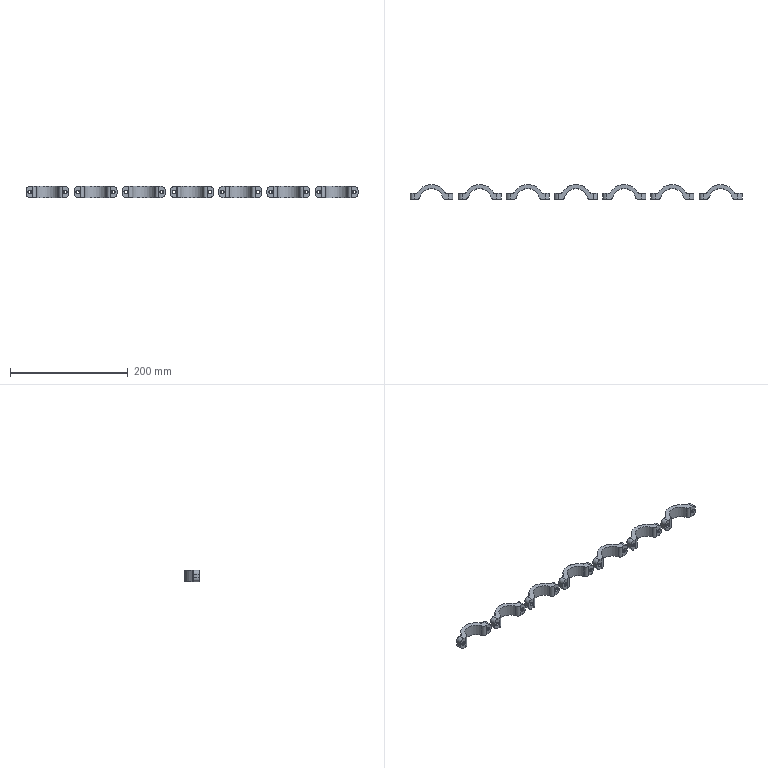NC program | Mastercam | posted with a generic post
Lines 1 to 18 of 23883:
%
:0001()
(MATERIAL - ALUMINUM MM - 2024)
(T1|16 CO |H1|XY STOCK TO LEAVE - 3.5|Z STOCK TO LEAVE - 0.)
(T2|8 FI |H2|D2|WEAR COMP|TOOL DIA. - 8.|XY STOCK TO LEAVE - .05|Z STOCK TO LEAVE - 0.)
(T3|6R0.5 MI |H3)
(T4|6 CHM |H4|D4|WEAR COMP|TOOL DIA. - 6.)
(T9|4 BM |H9)
(T6|5 DR |H6)
(T8|6.8 DR |H8)
(T7|M6 X 1 RH |H7)
(T5|8 FEMR |H5)
(T10|8 DR |H10)
(T11|6 FEM |H11|XY STOCK TO LEAVE - .15|Z STOCK TO LEAVE - .1)
N100 G21
N102 G0 G17 G40 G80 G90 G94 G98
N104 G0 G28 G91 Z0.
N106 G0 G28 X0. Y0.